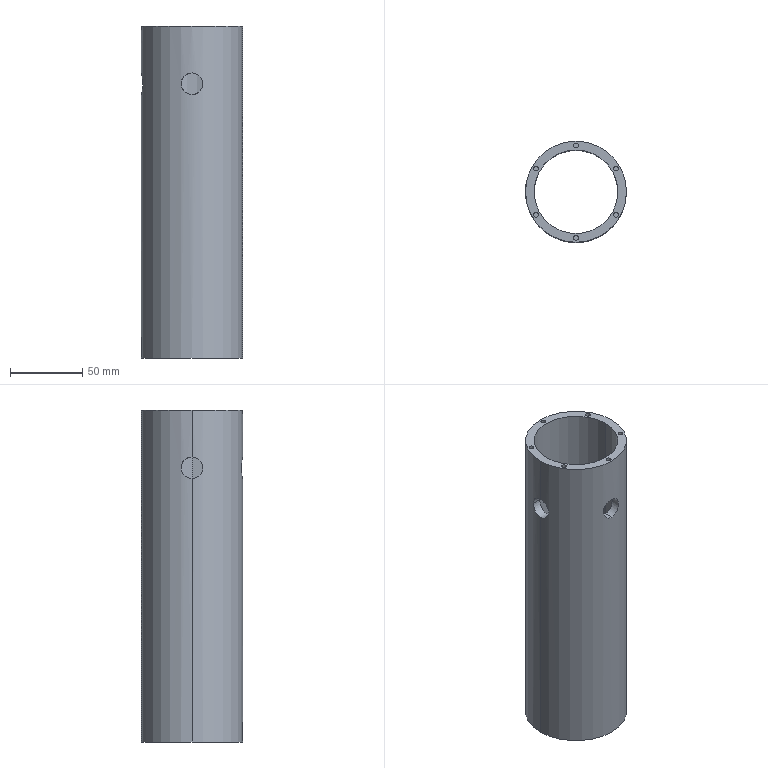Part | STEP file | Connecting tube sleeve | 1 solid | 40 faces | box 70 x 70 x 230 mm | volume 273867 mm3 | cylinder 28 | plane 12 | commonest cylinder face diameters 3.3 x20 15 x4 58 x2 70 x2